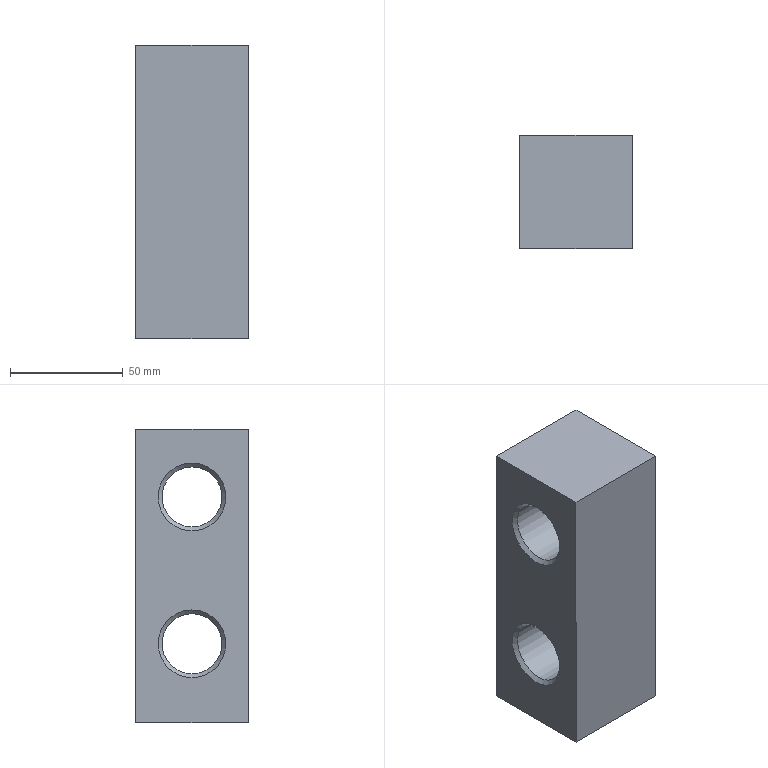Part | NX | features DATUM_CSYS 3, SIMPLE HOLE 2, SKETCH 2, SYMBOLIC_THREAD 2, EXTRUDE 1, HOLE PACKAGE 1 | 1 solid | 12 faces | box 50 x 50 x 130 mm | volume 268964 mm3 | plane 6 | cone 4 | cylinder 2 | commonest cylinder face diameters 26.59 x2
STEP:
#1=CARTESIAN_POINT('',(0.,-25.,65.));
#2=VERTEX_POINT('',#1);
#3=CARTESIAN_POINT('',(0.,-25.,-65.));
#4=VERTEX_POINT('',#3);
#5=CARTESIAN_POINT('',(0.,-25.,65.));
#6=DIRECTION('',(0.,0.,-1.));
#7=VECTOR('',#6,1000.);
#8=LINE('',#5,#7);
#9=EDGE_CURVE('',#2,#4,#8,.T.);
#10=ORIENTED_EDGE('',*,*,#9,.T.);
#11=CARTESIAN_POINT('',(50.,-25.,-65.));
#12=VERTEX_POINT('',#11);
#13=CARTESIAN_POINT('',(50.,-25.,-65.));
#14=DIRECTION('',(-1.,0.,0.));
#15=VECTOR('',#14,1000.);
#16=LINE('',#13,#15);
#17=EDGE_CURVE('',#12,#4,#16,.T.);
#18=ORIENTED_EDGE('',*,*,#17,.F.);
#19=CARTESIAN_POINT('',(50.,-25.,65.));
#20=VERTEX_POINT('',#19);
#21=CARTESIAN_POINT('',(50.,-25.,65.));
#22=DIRECTION('',(0.,0.,-1.));
#23=VECTOR('',#22,1000.);
#24=LINE('',#21,#23);
#25=EDGE_CURVE('',#20,#12,#24,.T.);
#26=ORIENTED_EDGE('',*,*,#25,.F.);
#27=CARTESIAN_POINT('',(50.,-25.,65.));
#28=DIRECTION('',(-1.,0.,0.));
#29=VECTOR('',#28,1000.);
#30=LINE('',#27,#29);
#31=EDGE_CURVE('',#20,#2,#30,.T.);
#32=ORIENTED_EDGE('',*,*,#31,.T.);
#33=EDGE_LOOP('',(#10,#18,#26,#32));
#34=FACE_BOUND('',#33,.T.);
#35=CARTESIAN_POINT('',(50.,-25.,65.));
#36=DIRECTION('',(0.,1.,0.));
#37=DIRECTION('',(0.,0.,1.));
#38=AXIS2_PLACEMENT_3D('',#35,#36,#37);
#39=PLANE('',#38);
#40=ADVANCED_FACE('',(#34),#39,.F.);
#41=CARTESIAN_POINT('',(0.,25.,-65.));
#42=VERTEX_POINT('',#41);
#43=CARTESIAN_POINT('',(0.,-25.,-65.));
#44=DIRECTION('',(0.,1.,0.));
#45=VECTOR('',#44,1000.);
#46=LINE('',#43,#45);
#47=EDGE_CURVE('',#4,#42,#46,.T.);
#48=ORIENTED_EDGE('',*,*,#47,.T.);
#49=CARTESIAN_POINT('',(50.,25.,-65.));
#50=VERTEX_POINT('',#49);
#51=CARTESIAN_POINT('',(50.,25.,-65.));
#52=DIRECTION('',(-1.,0.,0.));
#53=VECTOR('',#52,1000.);
#54=LINE('',#51,#53);
#55=EDGE_CURVE('',#50,#42,#54,.T.);
#56=ORIENTED_EDGE('',*,*,#55,.F.);
#57=CARTESIAN_POINT('',(50.,-25.,-65.));
#58=DIRECTION('',(0.,1.,0.));
#59=VECTOR('',#58,1000.);
#60=LINE('',#57,#59);
#61=EDGE_CURVE('',#12,#50,#60,.T.);
#62=ORIENTED_EDGE('',*,*,#61,.F.);
#63=ORIENTED_EDGE('',*,*,#17,.T.);
#64=EDGE_LOOP('',(#48,#56,#62,#63));
#65=FACE_BOUND('',#64,.T.);
#66=CARTESIAN_POINT('',(50.,-25.,-65.));
#67=DIRECTION('',(0.,0.,1.));
#68=DIRECTION('',(1.,0.,0.));
#69=AXIS2_PLACEMENT_3D('',#66,#67,#68);
#70=PLANE('',#69);
#71=ADVANCED_FACE('',(#65),#70,.F.);
#72=CARTESIAN_POINT('',(0.,25.,65.));
#73=VERTEX_POINT('',#72);
#74=CARTESIAN_POINT('',(0.,25.,-65.));
#75=DIRECTION('',(0.,0.,1.));
#76=VECTOR('',#75,1000.);
#77=LINE('',#74,#76);
#78=EDGE_CURVE('',#42,#73,#77,.T.);
#79=ORIENTED_EDGE('',*,*,#78,.T.);
#80=CARTESIAN_POINT('',(50.,25.,65.));
#81=VERTEX_POINT('',#80);
#82=CARTESIAN_POINT('',(50.,25.,65.));
#83=DIRECTION('',(-1.,0.,0.));
#84=VECTOR('',#83,1000.);
#85=LINE('',#82,#84);
#86=EDGE_CURVE('',#81,#73,#85,.T.);
#87=ORIENTED_EDGE('',*,*,#86,.F.);
#88=CARTESIAN_POINT('',(50.,25.,-65.));
#89=DIRECTION('',(0.,0.,1.));
#90=VECTOR('',#89,1000.);
#91=LINE('',#88,#90);
#92=EDGE_CURVE('',#50,#81,#91,.T.);
#93=ORIENTED_EDGE('',*,*,#92,.F.);
#94=ORIENTED_EDGE('',*,*,#55,.T.);
#95=EDGE_LOOP('',(#79,#87,#93,#94));
#96=FACE_BOUND('',#95,.T.);
#97=CARTESIAN_POINT('',(50.,25.,-65.));
#98=DIRECTION('',(0.,-1.,0.));
#99=DIRECTION('',(0.,0.,-1.));
#100=AXIS2_PLACEMENT_3D('',#97,#98,#99);
#101=PLANE('',#100);
#102=ADVANCED_FACE('',(#96),#101,.F.);
#103=CARTESIAN_POINT('',(0.,25.,65.));
#104=DIRECTION('',(0.,-1.,0.));
#105=VECTOR('',#104,1000.);
#106=LINE('',#103,#105);
#107=EDGE_CURVE('',#73,#2,#106,.T.);
#108=ORIENTED_EDGE('',*,*,#107,.T.);
#109=ORIENTED_EDGE('',*,*,#31,.F.);
#110=CARTESIAN_POINT('',(50.,25.,65.));
#111=DIRECTION('',(0.,-1.,0.));
#112=VECTOR('',#111,1000.);
#113=LINE('',#110,#112);
#114=EDGE_CURVE('',#81,#20,#113,.T.);
#115=ORIENTED_EDGE('',*,*,#114,.F.);
#116=ORIENTED_EDGE('',*,*,#86,.T.);
#117=EDGE_LOOP('',(#108,#109,#115,#116));
#118=FACE_BOUND('',#117,.T.);
#119=CARTESIAN_POINT('',(50.,25.,65.));
#120=DIRECTION('',(0.,0.,-1.));
#121=DIRECTION('',(-1.,0.,0.));
#122=AXIS2_PLACEMENT_3D('',#119,#120,#121);
#123=PLANE('',#122);
#124=ADVANCED_FACE('',(#118),#123,.F.);
#125=CARTESIAN_POINT('',(50.,0.,20.));
#126=VERTEX_POINT('',#125);
#127=CARTESIAN_POINT('',(50.,0.,35.));
#128=DIRECTION('',(1.,0.,0.));
#129=DIRECTION('',(0.,0.,-1.));
#130=AXIS2_PLACEMENT_3D('',#127,#128,#129);
#131=CIRCLE('',#130,15.);
#132=EDGE_CURVE('',#126,#126,#131,.F.);
#133=ORIENTED_EDGE('',*,*,#132,.T.);
#134=EDGE_LOOP('',(#133));
#135=FACE_BOUND('',#134,.T.);
#136=CARTESIAN_POINT('',(50.,0.,-45.));
#137=VERTEX_POINT('',#136);
#138=CARTESIAN_POINT('',(50.,0.,-30.));
#139=DIRECTION('',(1.,0.,0.));
#140=DIRECTION('',(0.,0.,-1.));
#141=AXIS2_PLACEMENT_3D('',#138,#139,#140);
#142=CIRCLE('',#141,15.);
#143=EDGE_CURVE('',#137,#137,#142,.F.);
#144=ORIENTED_EDGE('',*,*,#143,.T.);
#145=EDGE_LOOP('',(#144));
#146=FACE_BOUND('',#145,.T.);
#147=ORIENTED_EDGE('',*,*,#25,.T.);
#148=ORIENTED_EDGE('',*,*,#61,.T.);
#149=ORIENTED_EDGE('',*,*,#92,.T.);
#150=ORIENTED_EDGE('',*,*,#114,.T.);
#151=EDGE_LOOP('',(#147,#148,#149,#150));
#152=FACE_BOUND('',#151,.T.);
#153=CARTESIAN_POINT('',(50.,0.,0.));
#154=DIRECTION('',(1.,0.,0.));
#155=DIRECTION('',(0.,0.,-1.));
#156=AXIS2_PLACEMENT_3D('',#153,#154,#155);
#157=PLANE('',#156);
#158=ADVANCED_FACE('',(#135,#146,#152),#157,.T.);
#159=CARTESIAN_POINT('',(0.,0.,20.));
#160=VERTEX_POINT('',#159);
#161=CARTESIAN_POINT('',(0.,0.,35.));
#162=DIRECTION('',(1.,0.,0.));
#163=DIRECTION('',(0.,0.,-1.));
#164=AXIS2_PLACEMENT_3D('',#161,#162,#163);
#165=CIRCLE('',#164,15.);
#166=EDGE_CURVE('',#160,#160,#165,.T.);
#167=ORIENTED_EDGE('',*,*,#166,.T.);
#168=EDGE_LOOP('',(#167));
#169=FACE_BOUND('',#168,.T.);
#170=CARTESIAN_POINT('',(0.,0.,-45.));
#171=VERTEX_POINT('',#170);
#172=CARTESIAN_POINT('',(0.,0.,-30.));
#173=DIRECTION('',(1.,0.,0.));
#174=DIRECTION('',(0.,0.,-1.));
#175=AXIS2_PLACEMENT_3D('',#172,#173,#174);
#176=CIRCLE('',#175,15.);
#177=EDGE_CURVE('',#171,#171,#176,.T.);
#178=ORIENTED_EDGE('',*,*,#177,.T.);
#179=EDGE_LOOP('',(#178));
#180=FACE_BOUND('',#179,.T.);
#181=ORIENTED_EDGE('',*,*,#9,.F.);
#182=ORIENTED_EDGE('',*,*,#107,.F.);
#183=ORIENTED_EDGE('',*,*,#78,.F.);
#184=ORIENTED_EDGE('',*,*,#47,.F.);
#185=EDGE_LOOP('',(#181,#182,#183,#184));
#186=FACE_BOUND('',#185,.T.);
#187=CARTESIAN_POINT('',(0.,0.,0.));
#188=DIRECTION('',(1.,0.,0.));
#189=DIRECTION('',(0.,0.,-1.));
#190=AXIS2_PLACEMENT_3D('',#187,#188,#189);
#191=PLANE('',#190);
#192=ADVANCED_FACE('',(#169,#180,#186),#191,.F.);
#193=CARTESIAN_POINT('',(1.705,0.,-43.295));
#194=VERTEX_POINT('',#193);
#195=CARTESIAN_POINT('',(1.705,0.,-30.));
#196=DIRECTION('',(1.,0.,0.));
#197=DIRECTION('',(0.,0.,-1.));
#198=AXIS2_PLACEMENT_3D('',#195,#196,#197);
#199=CIRCLE('',#198,13.295);
#200=EDGE_CURVE('',#194,#194,#199,.F.);
#201=ORIENTED_EDGE('',*,*,#200,.T.);
#202=EDGE_LOOP('',(#201));
#203=FACE_BOUND('',#202,.T.);
#204=CARTESIAN_POINT('',(48.295,0.,-43.295));
#205=VERTEX_POINT('',#204);
#206=CARTESIAN_POINT('',(48.295,0.,-30.));
#207=DIRECTION('',(1.,0.,0.));
#208=DIRECTION('',(0.,0.,-1.));
#209=AXIS2_PLACEMENT_3D('',#206,#207,#208);
#210=CIRCLE('',#209,13.295);
#211=EDGE_CURVE('',#205,#205,#210,.T.);
#212=ORIENTED_EDGE('',*,*,#211,.T.);
#213=EDGE_LOOP('',(#212));
#214=FACE_BOUND('',#213,.T.);
#215=CARTESIAN_POINT('',(50.,0.,-30.));
#216=DIRECTION('',(-1.,0.,0.));
#217=DIRECTION('',(0.,0.,1.));
#218=AXIS2_PLACEMENT_3D('',#215,#216,#217);
#219=CYLINDRICAL_SURFACE('',#218,13.295);
#220=ADVANCED_FACE('',(#203,#214),#219,.F.);
#221=ORIENTED_EDGE('',*,*,#211,.F.);
#222=EDGE_LOOP('',(#221));
#223=FACE_BOUND('',#222,.T.);
#224=ORIENTED_EDGE('',*,*,#143,.F.);
#225=EDGE_LOOP('',(#224));
#226=FACE_BOUND('',#225,.T.);
#227=CARTESIAN_POINT('',(50.,0.,-30.));
#228=DIRECTION('',(1.,0.,0.));
#229=DIRECTION('',(0.,0.,-1.));
#230=AXIS2_PLACEMENT_3D('',#227,#228,#229);
#231=CONICAL_SURFACE('',#230,15.,0.7854);
#232=ADVANCED_FACE('',(#223,#226),#231,.F.);
#233=ORIENTED_EDGE('',*,*,#200,.F.);
#234=EDGE_LOOP('',(#233));
#235=FACE_BOUND('',#234,.T.);
#236=ORIENTED_EDGE('',*,*,#177,.F.);
#237=EDGE_LOOP('',(#236));
#238=FACE_BOUND('',#237,.T.);
#239=CARTESIAN_POINT('',(0.,0.,-30.));
#240=DIRECTION('',(-1.,0.,0.));
#241=DIRECTION('',(0.,0.,1.));
#242=AXIS2_PLACEMENT_3D('',#239,#240,#241);
#243=CONICAL_SURFACE('',#242,15.,0.7854);
#244=ADVANCED_FACE('',(#235,#238),#243,.F.);
#245=CARTESIAN_POINT('',(1.705,0.,21.705));
#246=VERTEX_POINT('',#245);
#247=CARTESIAN_POINT('',(1.705,0.,35.));
#248=DIRECTION('',(1.,0.,0.));
#249=DIRECTION('',(0.,0.,-1.));
#250=AXIS2_PLACEMENT_3D('',#247,#248,#249);
#251=CIRCLE('',#250,13.295);
#252=EDGE_CURVE('',#246,#246,#251,.F.);
#253=ORIENTED_EDGE('',*,*,#252,.T.);
#254=EDGE_LOOP('',(#253));
#255=FACE_BOUND('',#254,.T.);
#256=CARTESIAN_POINT('',(48.295,0.,21.705));
#257=VERTEX_POINT('',#256);
#258=CARTESIAN_POINT('',(48.295,0.,35.));
#259=DIRECTION('',(1.,0.,0.));
#260=DIRECTION('',(0.,0.,-1.));
#261=AXIS2_PLACEMENT_3D('',#258,#259,#260);
#262=CIRCLE('',#261,13.295);
#263=EDGE_CURVE('',#257,#257,#262,.T.);
#264=ORIENTED_EDGE('',*,*,#263,.T.);
#265=EDGE_LOOP('',(#264));
#266=FACE_BOUND('',#265,.T.);
#267=CARTESIAN_POINT('',(50.,0.,35.));
#268=DIRECTION('',(-1.,0.,0.));
#269=DIRECTION('',(0.,0.,1.));
#270=AXIS2_PLACEMENT_3D('',#267,#268,#269);
#271=CYLINDRICAL_SURFACE('',#270,13.295);
#272=ADVANCED_FACE('',(#255,#266),#271,.F.);
#273=ORIENTED_EDGE('',*,*,#263,.F.);
#274=EDGE_LOOP('',(#273));
#275=FACE_BOUND('',#274,.T.);
#276=ORIENTED_EDGE('',*,*,#132,.F.);
#277=EDGE_LOOP('',(#276));
#278=FACE_BOUND('',#277,.T.);
#279=CARTESIAN_POINT('',(50.,0.,35.));
#280=DIRECTION('',(1.,0.,0.));
#281=DIRECTION('',(0.,0.,-1.));
#282=AXIS2_PLACEMENT_3D('',#279,#280,#281);
#283=CONICAL_SURFACE('',#282,15.,0.7854);
#284=ADVANCED_FACE('',(#275,#278),#283,.F.);
#285=ORIENTED_EDGE('',*,*,#252,.F.);
#286=EDGE_LOOP('',(#285));
#287=FACE_BOUND('',#286,.T.);
#288=ORIENTED_EDGE('',*,*,#166,.F.);
#289=EDGE_LOOP('',(#288));
#290=FACE_BOUND('',#289,.T.);
#291=CARTESIAN_POINT('',(0.,0.,35.));
#292=DIRECTION('',(-1.,0.,0.));
#293=DIRECTION('',(0.,0.,1.));
#294=AXIS2_PLACEMENT_3D('',#291,#292,#293);
#295=CONICAL_SURFACE('',#294,15.,0.7854);
#296=ADVANCED_FACE('',(#287,#290),#295,.F.);
#297=CLOSED_SHELL('',(#40,#71,#102,#124,#158,#192,#220,#232,#244,#272,#284,#296));
#298=MANIFOLD_SOLID_BREP('',#297);
#299=(LENGTH_UNIT()NAMED_UNIT(*)SI_UNIT(.MILLI.,.METRE.));
#300=UNCERTAINTY_MEASURE_WITH_UNIT(LENGTH_MEASURE(0.00001),#299,'','');
#301=(NAMED_UNIT(*)PLANE_ANGLE_UNIT()SI_UNIT($,.RADIAN.));
#302=(NAMED_UNIT(*)SI_UNIT($,.STERADIAN.)SOLID_ANGLE_UNIT());
#303=(GEOMETRIC_REPRESENTATION_CONTEXT(3)GLOBAL_UNCERTAINTY_ASSIGNED_CONTEXT((#300))GLOBAL_UNIT_ASSIGNED_CONTEXT((#299,#301,#302))REPRESENTATION_CONTEXT('',''));
#304=ADVANCED_BREP_SHAPE_REPRESENTATION('',(#298),#303);